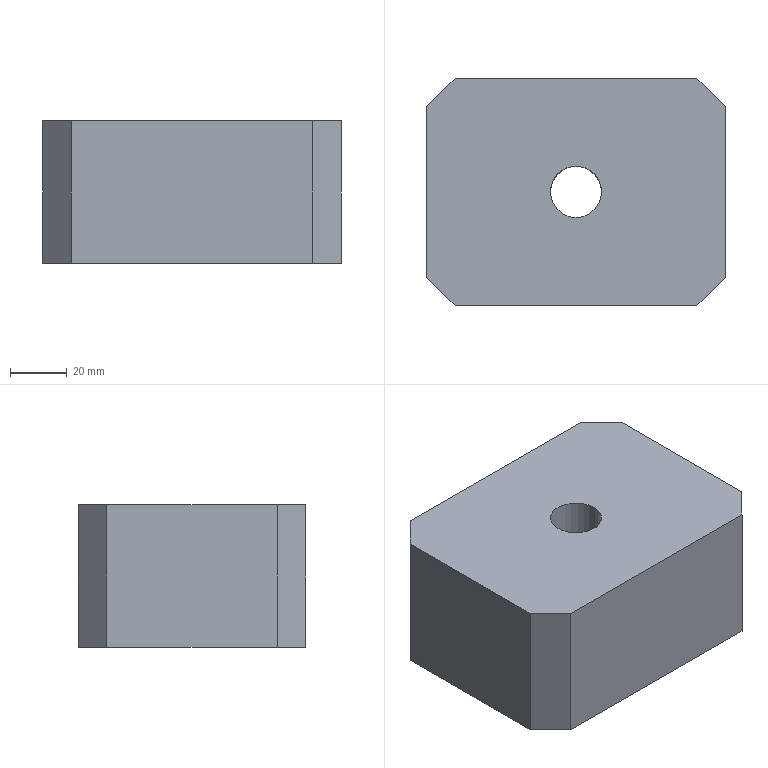Part | STEP file | [J453-EBZ05-16-00] | 1 solid | 12 faces | box 105 x 80 x 50 mm | volume 397277 mm3 | plane 10 | cylinder 2 | commonest cylinder face diameters 18 x2
STEP:
#1=CARTESIAN_POINT('',(0.,0.,0.));
#2=DIRECTION('',(0.,0.,1.));
#3=DIRECTION('',(1.,0.,0.));
#4=AXIS2_PLACEMENT_3D('',#1,#2,#3);
#5=CARTESIAN_POINT('',(61.5,40.,50.));
#6=VERTEX_POINT('',#5);
#7=CARTESIAN_POINT('',(61.5,40.,0.));
#8=VERTEX_POINT('',#7);
#9=CARTESIAN_POINT('',(61.5,40.,50.));
#10=DIRECTION('',(0.,0.,-1.));
#11=VECTOR('',#10,1.);
#12=LINE('',#9,#11);
#13=CARTESIAN_POINT('',(52.5,40.,50.));
#14=DIRECTION('',(0.,0.,-1.));
#15=DIRECTION('',(1.,0.,0.));
#16=AXIS2_PLACEMENT_3D('',#13,#14,#15);
#17=CYLINDRICAL_SURFACE('',#16,9.);
#18=CARTESIAN_POINT('',(6.283,0.));
#19=DIRECTION('',(0.,1.));
#20=VECTOR('',#19,1.);
#21=LINE('',#18,#20);
#22=(GEOMETRIC_REPRESENTATION_CONTEXT(2)PARAMETRIC_REPRESENTATION_CONTEXT()REPRESENTATION_CONTEXT('',''));
#23=DEFINITIONAL_REPRESENTATION('',(#21),#22);
#24=PCURVE('',#17,#23);
#25=CARTESIAN_POINT('',(52.5,40.,50.));
#26=DIRECTION('',(0.,0.,-1.));
#27=DIRECTION('',(1.,0.,0.));
#28=AXIS2_PLACEMENT_3D('',#25,#26,#27);
#29=CYLINDRICAL_SURFACE('',#28,9.);
#30=CARTESIAN_POINT('',(0.,0.));
#31=DIRECTION('',(0.,1.));
#32=VECTOR('',#31,1.);
#33=LINE('',#30,#32);
#34=(GEOMETRIC_REPRESENTATION_CONTEXT(2)PARAMETRIC_REPRESENTATION_CONTEXT()REPRESENTATION_CONTEXT('',''));
#35=DEFINITIONAL_REPRESENTATION('',(#33),#34);
#36=PCURVE('',#29,#35);
#37=SURFACE_CURVE('',#12,(#24,#36),.PCURVE_S1.);
#38=EDGE_CURVE('',#6,#8,#37,.T.);
#39=ORIENTED_EDGE('',*,*,#38,.T.);
#40=CARTESIAN_POINT('',(43.5,40.,0.));
#41=VERTEX_POINT('',#40);
#42=CARTESIAN_POINT('',(52.5,40.,0.));
#43=DIRECTION('',(0.,0.,1.));
#44=DIRECTION('',(-1.,0.,0.));
#45=AXIS2_PLACEMENT_3D('',#42,#43,#44);
#46=CIRCLE('',#45,9.);
#47=CARTESIAN_POINT('',(9.425,50.));
#48=DIRECTION('',(-1.,0.));
#49=VECTOR('',#48,1.);
#50=LINE('',#47,#49);
#51=(GEOMETRIC_REPRESENTATION_CONTEXT(2)PARAMETRIC_REPRESENTATION_CONTEXT()REPRESENTATION_CONTEXT('',''));
#52=DEFINITIONAL_REPRESENTATION('',(#50),#51);
#53=PCURVE('',#17,#52);
#54=CARTESIAN_POINT('',(0.,40.,0.));
#55=DIRECTION('',(0.,0.,-1.));
#56=DIRECTION('',(1.,0.,0.));
#57=AXIS2_PLACEMENT_3D('',#54,#55,#56);
#58=PLANE('',#57);
#59=CARTESIAN_POINT('',(43.5,0.));
#60=CARTESIAN_POINT('',(43.5,15.588));
#61=CARTESIAN_POINT('',(57.,7.794));
#62=CARTESIAN_POINT('',(70.5,0.));
#63=CARTESIAN_POINT('',(57.,-7.794));
#64=CARTESIAN_POINT('',(43.5,-15.588));
#65=CARTESIAN_POINT('',(43.5,0.));
#66=(BOUNDED_CURVE()B_SPLINE_CURVE(2,(#59,#60,#61,#62,#63,#64,#65),.UNSPECIFIED.,.T.,.F.)B_SPLINE_CURVE_WITH_KNOTS((1,2,2,2,2,1),(-2.094,0.,2.094,4.189,6.283,8.378),.UNSPECIFIED.)CURVE()GEOMETRIC_REPRESENTATION_ITEM()RATIONAL_B_SPLINE_CURVE((1.,0.5,1.,0.5,1.,0.5,1.))REPRESENTATION_ITEM(''));
#67=(GEOMETRIC_REPRESENTATION_CONTEXT(2)PARAMETRIC_REPRESENTATION_CONTEXT()REPRESENTATION_CONTEXT('',''));
#68=DEFINITIONAL_REPRESENTATION('',(#66),#67);
#69=PCURVE('',#58,#68);
#70=SURFACE_CURVE('',#46,(#53,#69),.PCURVE_S1.);
#71=EDGE_CURVE('',#8,#41,#70,.T.);
#72=ORIENTED_EDGE('',*,*,#71,.T.);
#73=CARTESIAN_POINT('',(43.5,40.,50.));
#74=VERTEX_POINT('',#73);
#75=CARTESIAN_POINT('',(43.5,40.,50.));
#76=DIRECTION('',(0.,0.,-1.));
#77=VECTOR('',#76,1.);
#78=LINE('',#75,#77);
#79=CARTESIAN_POINT('',(3.142,0.));
#80=DIRECTION('',(0.,1.));
#81=VECTOR('',#80,1.);
#82=LINE('',#79,#81);
#83=(GEOMETRIC_REPRESENTATION_CONTEXT(2)PARAMETRIC_REPRESENTATION_CONTEXT()REPRESENTATION_CONTEXT('',''));
#84=DEFINITIONAL_REPRESENTATION('',(#82),#83);
#85=PCURVE('',#17,#84);
#86=CARTESIAN_POINT('',(3.142,0.));
#87=DIRECTION('',(0.,1.));
#88=VECTOR('',#87,1.);
#89=LINE('',#86,#88);
#90=(GEOMETRIC_REPRESENTATION_CONTEXT(2)PARAMETRIC_REPRESENTATION_CONTEXT()REPRESENTATION_CONTEXT('',''));
#91=DEFINITIONAL_REPRESENTATION('',(#89),#90);
#92=PCURVE('',#29,#91);
#93=SURFACE_CURVE('',#78,(#85,#92),.PCURVE_S1.);
#94=EDGE_CURVE('',#74,#41,#93,.T.);
#95=ORIENTED_EDGE('',*,*,#94,.F.);
#96=CARTESIAN_POINT('',(52.5,40.,50.));
#97=DIRECTION('',(0.,0.,-1.));
#98=DIRECTION('',(1.,0.,0.));
#99=AXIS2_PLACEMENT_3D('',#96,#97,#98);
#100=CIRCLE('',#99,9.);
#101=CARTESIAN_POINT('',(0.,0.));
#102=DIRECTION('',(1.,0.));
#103=VECTOR('',#102,1.);
#104=LINE('',#101,#103);
#105=(GEOMETRIC_REPRESENTATION_CONTEXT(2)PARAMETRIC_REPRESENTATION_CONTEXT()REPRESENTATION_CONTEXT('',''));
#106=DEFINITIONAL_REPRESENTATION('',(#104),#105);
#107=PCURVE('',#17,#106);
#108=CARTESIAN_POINT('',(0.,40.,50.));
#109=DIRECTION('',(0.,0.,1.));
#110=DIRECTION('',(-1.,0.,0.));
#111=AXIS2_PLACEMENT_3D('',#108,#109,#110);
#112=PLANE('',#111);
#113=CARTESIAN_POINT('',(-61.5,0.));
#114=CARTESIAN_POINT('',(-61.5,15.588));
#115=CARTESIAN_POINT('',(-48.,7.794));
#116=CARTESIAN_POINT('',(-34.5,0.));
#117=CARTESIAN_POINT('',(-48.,-7.794));
#118=CARTESIAN_POINT('',(-61.5,-15.588));
#119=CARTESIAN_POINT('',(-61.5,0.));
#120=(BOUNDED_CURVE()B_SPLINE_CURVE(2,(#113,#114,#115,#116,#117,#118,#119),.UNSPECIFIED.,.T.,.F.)B_SPLINE_CURVE_WITH_KNOTS((1,2,2,2,2,1),(-2.094,0.,2.094,4.189,6.283,8.378),.UNSPECIFIED.)CURVE()GEOMETRIC_REPRESENTATION_ITEM()RATIONAL_B_SPLINE_CURVE((1.,0.5,1.,0.5,1.,0.5,1.))REPRESENTATION_ITEM(''));
#121=(GEOMETRIC_REPRESENTATION_CONTEXT(2)PARAMETRIC_REPRESENTATION_CONTEXT()REPRESENTATION_CONTEXT('',''));
#122=DEFINITIONAL_REPRESENTATION('',(#120),#121);
#123=PCURVE('',#112,#122);
#124=SURFACE_CURVE('',#100,(#107,#123),.PCURVE_S1.);
#125=EDGE_CURVE('',#74,#6,#124,.T.);
#126=ORIENTED_EDGE('',*,*,#125,.T.);
#127=EDGE_LOOP('',(#39,#72,#95,#126));
#128=FACE_BOUND('',#127,.F.);
#129=ADVANCED_FACE('',(#128),#17,.F.);
#130=CARTESIAN_POINT('',(105.,70.,0.));
#131=VERTEX_POINT('',#130);
#132=CARTESIAN_POINT('',(105.,10.,0.));
#133=VERTEX_POINT('',#132);
#134=CARTESIAN_POINT('',(105.,40.,0.));
#135=DIRECTION('',(0.,-1.,0.));
#136=VECTOR('',#135,1.);
#137=LINE('',#134,#136);
#138=CARTESIAN_POINT('',(105.,40.,25.));
#139=DIRECTION('',(1.,0.,0.));
#140=DIRECTION('',(0.,0.,1.));
#141=AXIS2_PLACEMENT_3D('',#138,#139,#140);
#142=PLANE('',#141);
#143=CARTESIAN_POINT('',(-25.,0.));
#144=DIRECTION('',(0.,1.));
#145=VECTOR('',#144,1.);
#146=LINE('',#143,#145);
#147=(GEOMETRIC_REPRESENTATION_CONTEXT(2)PARAMETRIC_REPRESENTATION_CONTEXT()REPRESENTATION_CONTEXT('',''));
#148=DEFINITIONAL_REPRESENTATION('',(#146),#147);
#149=PCURVE('',#142,#148);
#150=CARTESIAN_POINT('',(105.,0.));
#151=DIRECTION('',(0.,1.));
#152=VECTOR('',#151,1.);
#153=LINE('',#150,#152);
#154=(GEOMETRIC_REPRESENTATION_CONTEXT(2)PARAMETRIC_REPRESENTATION_CONTEXT()REPRESENTATION_CONTEXT('',''));
#155=DEFINITIONAL_REPRESENTATION('',(#153),#154);
#156=PCURVE('',#58,#155);
#157=SURFACE_CURVE('',#137,(#149,#156),.PCURVE_S1.);
#158=EDGE_CURVE('',#131,#133,#157,.T.);
#159=ORIENTED_EDGE('',*,*,#158,.F.);
#160=CARTESIAN_POINT('',(105.,70.,50.));
#161=VERTEX_POINT('',#160);
#162=CARTESIAN_POINT('',(105.,70.,25.));
#163=DIRECTION('',(0.,0.,1.));
#164=VECTOR('',#163,1.);
#165=LINE('',#162,#164);
#166=CARTESIAN_POINT('',(0.,-30.));
#167=DIRECTION('',(1.,0.));
#168=VECTOR('',#167,1.);
#169=LINE('',#166,#168);
#170=(GEOMETRIC_REPRESENTATION_CONTEXT(2)PARAMETRIC_REPRESENTATION_CONTEXT()REPRESENTATION_CONTEXT('',''));
#171=DEFINITIONAL_REPRESENTATION('',(#169),#170);
#172=PCURVE('',#142,#171);
#173=CARTESIAN_POINT('',(95.,80.,25.));
#174=DIRECTION('',(-0.7071,-0.7071,0.));
#175=DIRECTION('',(0.,0.,-1.));
#176=AXIS2_PLACEMENT_3D('',#173,#174,#175);
#177=PLANE('',#176);
#178=CARTESIAN_POINT('',(0.,14.142));
#179=DIRECTION('',(-1.,0.));
#180=VECTOR('',#179,1.);
#181=LINE('',#178,#180);
#182=(GEOMETRIC_REPRESENTATION_CONTEXT(2)PARAMETRIC_REPRESENTATION_CONTEXT()REPRESENTATION_CONTEXT('',''));
#183=DEFINITIONAL_REPRESENTATION('',(#181),#182);
#184=PCURVE('',#177,#183);
#185=SURFACE_CURVE('',#165,(#172,#184),.PCURVE_S1.);
#186=EDGE_CURVE('',#131,#161,#185,.T.);
#187=ORIENTED_EDGE('',*,*,#186,.T.);
#188=CARTESIAN_POINT('',(105.,10.,50.));
#189=VERTEX_POINT('',#188);
#190=CARTESIAN_POINT('',(105.,40.,50.));
#191=DIRECTION('',(0.,1.,0.));
#192=VECTOR('',#191,1.);
#193=LINE('',#190,#192);
#194=CARTESIAN_POINT('',(25.,0.));
#195=DIRECTION('',(0.,-1.));
#196=VECTOR('',#195,1.);
#197=LINE('',#194,#196);
#198=(GEOMETRIC_REPRESENTATION_CONTEXT(2)PARAMETRIC_REPRESENTATION_CONTEXT()REPRESENTATION_CONTEXT('',''));
#199=DEFINITIONAL_REPRESENTATION('',(#197),#198);
#200=PCURVE('',#142,#199);
#201=CARTESIAN_POINT('',(-105.,0.));
#202=DIRECTION('',(0.,-1.));
#203=VECTOR('',#202,1.);
#204=LINE('',#201,#203);
#205=(GEOMETRIC_REPRESENTATION_CONTEXT(2)PARAMETRIC_REPRESENTATION_CONTEXT()REPRESENTATION_CONTEXT('',''));
#206=DEFINITIONAL_REPRESENTATION('',(#204),#205);
#207=PCURVE('',#112,#206);
#208=SURFACE_CURVE('',#193,(#200,#207),.PCURVE_S1.);
#209=EDGE_CURVE('',#189,#161,#208,.T.);
#210=ORIENTED_EDGE('',*,*,#209,.F.);
#211=CARTESIAN_POINT('',(105.,10.,25.));
#212=DIRECTION('',(0.,0.,-1.));
#213=VECTOR('',#212,1.);
#214=LINE('',#211,#213);
#215=CARTESIAN_POINT('',(0.,30.));
#216=DIRECTION('',(-1.,0.));
#217=VECTOR('',#216,1.);
#218=LINE('',#215,#217);
#219=(GEOMETRIC_REPRESENTATION_CONTEXT(2)PARAMETRIC_REPRESENTATION_CONTEXT()REPRESENTATION_CONTEXT('',''));
#220=DEFINITIONAL_REPRESENTATION('',(#218),#219);
#221=PCURVE('',#142,#220);
#222=CARTESIAN_POINT('',(95.,0.,25.));
#223=DIRECTION('',(-0.7071,0.7071,0.));
#224=DIRECTION('',(0.,0.,1.));
#225=AXIS2_PLACEMENT_3D('',#222,#223,#224);
#226=PLANE('',#225);
#227=CARTESIAN_POINT('',(0.,14.142));
#228=DIRECTION('',(-1.,0.));
#229=VECTOR('',#228,1.);
#230=LINE('',#227,#229);
#231=(GEOMETRIC_REPRESENTATION_CONTEXT(2)PARAMETRIC_REPRESENTATION_CONTEXT()REPRESENTATION_CONTEXT('',''));
#232=DEFINITIONAL_REPRESENTATION('',(#230),#231);
#233=PCURVE('',#226,#232);
#234=SURFACE_CURVE('',#214,(#221,#233),.PCURVE_S1.);
#235=EDGE_CURVE('',#189,#133,#234,.T.);
#236=ORIENTED_EDGE('',*,*,#235,.T.);
#237=EDGE_LOOP('',(#159,#187,#210,#236));
#238=FACE_BOUND('',#237,.T.);
#239=ADVANCED_FACE('',(#238),#142,.T.);
#240=CARTESIAN_POINT('',(10.,80.,50.));
#241=VERTEX_POINT('',#240);
#242=CARTESIAN_POINT('',(95.,80.,50.));
#243=VERTEX_POINT('',#242);
#244=CARTESIAN_POINT('',(0.,80.,50.));
#245=DIRECTION('',(1.,0.,0.));
#246=VECTOR('',#245,1.);
#247=LINE('',#244,#246);
#248=CARTESIAN_POINT('',(0.,80.,25.));
#249=DIRECTION('',(0.,1.,0.));
#250=DIRECTION('',(-1.,0.,0.));
#251=AXIS2_PLACEMENT_3D('',#248,#249,#250);
#252=PLANE('',#251);
#253=CARTESIAN_POINT('',(0.,25.));
#254=DIRECTION('',(-1.,0.));
#255=VECTOR('',#254,1.);
#256=LINE('',#253,#255);
#257=(GEOMETRIC_REPRESENTATION_CONTEXT(2)PARAMETRIC_REPRESENTATION_CONTEXT()REPRESENTATION_CONTEXT('',''));
#258=DEFINITIONAL_REPRESENTATION('',(#256),#257);
#259=PCURVE('',#252,#258);
#260=CARTESIAN_POINT('',(0.,-40.));
#261=DIRECTION('',(-1.,0.));
#262=VECTOR('',#261,1.);
#263=LINE('',#260,#262);
#264=(GEOMETRIC_REPRESENTATION_CONTEXT(2)PARAMETRIC_REPRESENTATION_CONTEXT()REPRESENTATION_CONTEXT('',''));
#265=DEFINITIONAL_REPRESENTATION('',(#263),#264);
#266=PCURVE('',#112,#265);
#267=SURFACE_CURVE('',#247,(#259,#266),.PCURVE_S1.);
#268=EDGE_CURVE('',#241,#243,#267,.T.);
#269=ORIENTED_EDGE('',*,*,#268,.T.);
#270=CARTESIAN_POINT('',(95.,80.,0.));
#271=VERTEX_POINT('',#270);
#272=CARTESIAN_POINT('',(95.,80.,25.));
#273=DIRECTION('',(0.,0.,-1.));
#274=VECTOR('',#273,1.);
#275=LINE('',#272,#274);
#276=CARTESIAN_POINT('',(-95.,0.));
#277=DIRECTION('',(0.,-1.));
#278=VECTOR('',#277,1.);
#279=LINE('',#276,#278);
#280=(GEOMETRIC_REPRESENTATION_CONTEXT(2)PARAMETRIC_REPRESENTATION_CONTEXT()REPRESENTATION_CONTEXT('',''));
#281=DEFINITIONAL_REPRESENTATION('',(#279),#280);
#282=PCURVE('',#252,#281);
#283=CARTESIAN_POINT('',(0.,0.));
#284=DIRECTION('',(1.,0.));
#285=VECTOR('',#284,1.);
#286=LINE('',#283,#285);
#287=(GEOMETRIC_REPRESENTATION_CONTEXT(2)PARAMETRIC_REPRESENTATION_CONTEXT()REPRESENTATION_CONTEXT('',''));
#288=DEFINITIONAL_REPRESENTATION('',(#286),#287);
#289=PCURVE('',#177,#288);
#290=SURFACE_CURVE('',#275,(#282,#289),.PCURVE_S1.);
#291=EDGE_CURVE('',#243,#271,#290,.T.);
#292=ORIENTED_EDGE('',*,*,#291,.T.);
#293=CARTESIAN_POINT('',(10.,80.,0.));
#294=VERTEX_POINT('',#293);
#295=CARTESIAN_POINT('',(0.,80.,0.));
#296=DIRECTION('',(1.,0.,0.));
#297=VECTOR('',#296,1.);
#298=LINE('',#295,#297);
#299=CARTESIAN_POINT('',(0.,-25.));
#300=DIRECTION('',(-1.,0.));
#301=VECTOR('',#300,1.);
#302=LINE('',#299,#301);
#303=(GEOMETRIC_REPRESENTATION_CONTEXT(2)PARAMETRIC_REPRESENTATION_CONTEXT()REPRESENTATION_CONTEXT('',''));
#304=DEFINITIONAL_REPRESENTATION('',(#302),#303);
#305=PCURVE('',#252,#304);
#306=CARTESIAN_POINT('',(0.,-40.));
#307=DIRECTION('',(1.,0.));
#308=VECTOR('',#307,1.);
#309=LINE('',#306,#308);
#310=(GEOMETRIC_REPRESENTATION_CONTEXT(2)PARAMETRIC_REPRESENTATION_CONTEXT()REPRESENTATION_CONTEXT('',''));
#311=DEFINITIONAL_REPRESENTATION('',(#309),#310);
#312=PCURVE('',#58,#311);
#313=SURFACE_CURVE('',#298,(#305,#312),.PCURVE_S1.);
#314=EDGE_CURVE('',#294,#271,#313,.T.);
#315=ORIENTED_EDGE('',*,*,#314,.F.);
#316=CARTESIAN_POINT('',(10.,80.,25.));
#317=DIRECTION('',(0.,0.,1.));
#318=VECTOR('',#317,1.);
#319=LINE('',#316,#318);
#320=CARTESIAN_POINT('',(-10.,0.));
#321=DIRECTION('',(0.,1.));
#322=VECTOR('',#321,1.);
#323=LINE('',#320,#322);
#324=(GEOMETRIC_REPRESENTATION_CONTEXT(2)PARAMETRIC_REPRESENTATION_CONTEXT()REPRESENTATION_CONTEXT('',''));
#325=DEFINITIONAL_REPRESENTATION('',(#323),#324);
#326=PCURVE('',#252,#325);
#327=CARTESIAN_POINT('',(10.,80.,25.));
#328=DIRECTION('',(0.7071,-0.7071,0.));
#329=DIRECTION('',(0.,0.,1.));
#330=AXIS2_PLACEMENT_3D('',#327,#328,#329);
#331=PLANE('',#330);
#332=CARTESIAN_POINT('',(0.,0.));
#333=DIRECTION('',(1.,0.));
#334=VECTOR('',#333,1.);
#335=LINE('',#332,#334);
#336=(GEOMETRIC_REPRESENTATION_CONTEXT(2)PARAMETRIC_REPRESENTATION_CONTEXT()REPRESENTATION_CONTEXT('',''));
#337=DEFINITIONAL_REPRESENTATION('',(#335),#336);
#338=PCURVE('',#331,#337);
#339=SURFACE_CURVE('',#319,(#326,#338),.PCURVE_S1.);
#340=EDGE_CURVE('',#294,#241,#339,.T.);
#341=ORIENTED_EDGE('',*,*,#340,.T.);
#342=EDGE_LOOP('',(#269,#292,#315,#341));
#343=FACE_BOUND('',#342,.T.);
#344=ADVANCED_FACE('',(#343),#252,.T.);
#345=ORIENTED_EDGE('',*,*,#71,.T.);
#346=CARTESIAN_POINT('',(52.5,40.,0.));
#347=DIRECTION('',(0.,0.,1.));
#348=DIRECTION('',(-1.,0.,0.));
#349=AXIS2_PLACEMENT_3D('',#346,#347,#348);
#350=CIRCLE('',#349,9.);
#351=CARTESIAN_POINT('',(43.5,0.));
#352=CARTESIAN_POINT('',(43.5,15.588));
#353=CARTESIAN_POINT('',(57.,7.794));
#354=CARTESIAN_POINT('',(70.5,0.));
#355=CARTESIAN_POINT('',(57.,-7.794));
#356=CARTESIAN_POINT('',(43.5,-15.588));
#357=CARTESIAN_POINT('',(43.5,0.));
#358=(BOUNDED_CURVE()B_SPLINE_CURVE(2,(#351,#352,#353,#354,#355,#356,#357),.UNSPECIFIED.,.T.,.F.)B_SPLINE_CURVE_WITH_KNOTS((1,2,2,2,2,1),(-2.094,0.,2.094,4.189,6.283,8.378),.UNSPECIFIED.)CURVE()GEOMETRIC_REPRESENTATION_ITEM()RATIONAL_B_SPLINE_CURVE((1.,0.5,1.,0.5,1.,0.5,1.))REPRESENTATION_ITEM(''));
#359=(GEOMETRIC_REPRESENTATION_CONTEXT(2)PARAMETRIC_REPRESENTATION_CONTEXT()REPRESENTATION_CONTEXT('',''));
#360=DEFINITIONAL_REPRESENTATION('',(#358),#359);
#361=PCURVE('',#58,#360);
#362=CARTESIAN_POINT('',(3.142,50.));
#363=DIRECTION('',(-1.,0.));
#364=VECTOR('',#363,1.);
#365=LINE('',#362,#364);
#366=(GEOMETRIC_REPRESENTATION_CONTEXT(2)PARAMETRIC_REPRESENTATION_CONTEXT()REPRESENTATION_CONTEXT('',''));
#367=DEFINITIONAL_REPRESENTATION('',(#365),#366);
#368=PCURVE('',#29,#367);
#369=SURFACE_CURVE('',#350,(#361,#368),.PCURVE_S1.);
#370=EDGE_CURVE('',#41,#8,#369,.T.);
#371=ORIENTED_EDGE('',*,*,#370,.T.);
#372=EDGE_LOOP('',(#345,#371));
#373=FACE_BOUND('',#372,.T.);
#374=ORIENTED_EDGE('',*,*,#314,.T.);
#375=CARTESIAN_POINT('',(67.5,107.5,0.));
#376=DIRECTION('',(0.7071,-0.7071,0.));
#377=VECTOR('',#376,1.);
#378=LINE('',#375,#377);
#379=CARTESIAN_POINT('',(67.5,-67.5));
#380=DIRECTION('',(0.7071,0.7071));
#381=VECTOR('',#380,1.);
#382=LINE('',#379,#381);
#383=(GEOMETRIC_REPRESENTATION_CONTEXT(2)PARAMETRIC_REPRESENTATION_CONTEXT()REPRESENTATION_CONTEXT('',''));
#384=DEFINITIONAL_REPRESENTATION('',(#382),#383);
#385=PCURVE('',#58,#384);
#386=CARTESIAN_POINT('',(25.,-38.891));
#387=DIRECTION('',(0.,1.));
#388=VECTOR('',#387,1.);
#389=LINE('',#386,#388);
#390=(GEOMETRIC_REPRESENTATION_CONTEXT(2)PARAMETRIC_REPRESENTATION_CONTEXT()REPRESENTATION_CONTEXT('',''));
#391=DEFINITIONAL_REPRESENTATION('',(#389),#390);
#392=PCURVE('',#177,#391);
#393=SURFACE_CURVE('',#378,(#385,#392),.PCURVE_S1.);
#394=EDGE_CURVE('',#271,#131,#393,.T.);
#395=ORIENTED_EDGE('',*,*,#394,.T.);
#396=ORIENTED_EDGE('',*,*,#158,.T.);
#397=CARTESIAN_POINT('',(95.,0.,0.));
#398=VERTEX_POINT('',#397);
#399=CARTESIAN_POINT('',(67.5,-27.5,0.));
#400=DIRECTION('',(-0.7071,-0.7071,0.));
#401=VECTOR('',#400,1.);
#402=LINE('',#399,#401);
#403=CARTESIAN_POINT('',(67.5,67.5));
#404=DIRECTION('',(-0.7071,0.7071));
#405=VECTOR('',#404,1.);
#406=LINE('',#403,#405);
#407=(GEOMETRIC_REPRESENTATION_CONTEXT(2)PARAMETRIC_REPRESENTATION_CONTEXT()REPRESENTATION_CONTEXT('',''));
#408=DEFINITIONAL_REPRESENTATION('',(#406),#407);
#409=PCURVE('',#58,#408);
#410=CARTESIAN_POINT('',(-25.,-38.891));
#411=DIRECTION('',(0.,-1.));
#412=VECTOR('',#411,1.);
#413=LINE('',#410,#412);
#414=(GEOMETRIC_REPRESENTATION_CONTEXT(2)PARAMETRIC_REPRESENTATION_CONTEXT()REPRESENTATION_CONTEXT('',''));
#415=DEFINITIONAL_REPRESENTATION('',(#413),#414);
#416=PCURVE('',#226,#415);
#417=SURFACE_CURVE('',#402,(#409,#416),.PCURVE_S1.);
#418=EDGE_CURVE('',#133,#398,#417,.T.);
#419=ORIENTED_EDGE('',*,*,#418,.T.);
#420=CARTESIAN_POINT('',(10.,0.,0.));
#421=VERTEX_POINT('',#420);
#422=CARTESIAN_POINT('',(0.,0.,0.));
#423=DIRECTION('',(1.,0.,0.));
#424=VECTOR('',#423,1.);
#425=LINE('',#422,#424);
#426=CARTESIAN_POINT('',(0.,40.));
#427=DIRECTION('',(1.,0.));
#428=VECTOR('',#427,1.);
#429=LINE('',#426,#428);
#430=(GEOMETRIC_REPRESENTATION_CONTEXT(2)PARAMETRIC_REPRESENTATION_CONTEXT()REPRESENTATION_CONTEXT('',''));
#431=DEFINITIONAL_REPRESENTATION('',(#429),#430);
#432=PCURVE('',#58,#431);
#433=CARTESIAN_POINT('',(0.,0.,25.));
#434=DIRECTION('',(0.,-1.,0.));
#435=DIRECTION('',(1.,0.,0.));
#436=AXIS2_PLACEMENT_3D('',#433,#434,#435);
#437=PLANE('',#436);
#438=CARTESIAN_POINT('',(0.,-25.));
#439=DIRECTION('',(1.,0.));
#440=VECTOR('',#439,1.);
#441=LINE('',#438,#440);
#442=(GEOMETRIC_REPRESENTATION_CONTEXT(2)PARAMETRIC_REPRESENTATION_CONTEXT()REPRESENTATION_CONTEXT('',''));
#443=DEFINITIONAL_REPRESENTATION('',(#441),#442);
#444=PCURVE('',#437,#443);
#445=SURFACE_CURVE('',#425,(#432,#444),.PCURVE_S1.);
#446=EDGE_CURVE('',#421,#398,#445,.T.);
#447=ORIENTED_EDGE('',*,*,#446,.F.);
#448=CARTESIAN_POINT('',(0.,10.,0.));
#449=VERTEX_POINT('',#448);
#450=CARTESIAN_POINT('',(-15.,25.,0.));
#451=DIRECTION('',(-0.7071,0.7071,0.));
#452=VECTOR('',#451,1.);
#453=LINE('',#450,#452);
#454=CARTESIAN_POINT('',(-15.,15.));
#455=DIRECTION('',(-0.7071,-0.7071));
#456=VECTOR('',#455,1.);
#457=LINE('',#454,#456);
#458=(GEOMETRIC_REPRESENTATION_CONTEXT(2)PARAMETRIC_REPRESENTATION_CONTEXT()REPRESENTATION_CONTEXT('',''));
#459=DEFINITIONAL_REPRESENTATION('',(#457),#458);
#460=PCURVE('',#58,#459);
#461=CARTESIAN_POINT('',(10.,0.,25.));
#462=DIRECTION('',(0.7071,0.7071,0.));
#463=DIRECTION('',(0.,0.,-1.));
#464=AXIS2_PLACEMENT_3D('',#461,#462,#463);
#465=PLANE('',#464);
#466=CARTESIAN_POINT('',(25.,35.355));
#467=DIRECTION('',(0.,1.));
#468=VECTOR('',#467,1.);
#469=LINE('',#466,#468);
#470=(GEOMETRIC_REPRESENTATION_CONTEXT(2)PARAMETRIC_REPRESENTATION_CONTEXT()REPRESENTATION_CONTEXT('',''));
#471=DEFINITIONAL_REPRESENTATION('',(#469),#470);
#472=PCURVE('',#465,#471);
#473=SURFACE_CURVE('',#453,(#460,#472),.PCURVE_S1.);
#474=EDGE_CURVE('',#421,#449,#473,.T.);
#475=ORIENTED_EDGE('',*,*,#474,.T.);
#476=CARTESIAN_POINT('',(0.,70.,0.));
#477=VERTEX_POINT('',#476);
#478=CARTESIAN_POINT('',(0.,40.,0.));
#479=DIRECTION('',(0.,1.,0.));
#480=VECTOR('',#479,1.);
#481=LINE('',#478,#480);
#482=CARTESIAN_POINT('',(0.,0.));
#483=DIRECTION('',(0.,-1.));
#484=VECTOR('',#483,1.);
#485=LINE('',#482,#484);
#486=(GEOMETRIC_REPRESENTATION_CONTEXT(2)PARAMETRIC_REPRESENTATION_CONTEXT()REPRESENTATION_CONTEXT('',''));
#487=DEFINITIONAL_REPRESENTATION('',(#485),#486);
#488=PCURVE('',#58,#487);
#489=CARTESIAN_POINT('',(0.,40.,25.));
#490=DIRECTION('',(-1.,0.,0.));
#491=DIRECTION('',(0.,0.,-1.));
#492=AXIS2_PLACEMENT_3D('',#489,#490,#491);
#493=PLANE('',#492);
#494=CARTESIAN_POINT('',(25.,0.));
#495=DIRECTION('',(0.,-1.));
#496=VECTOR('',#495,1.);
#497=LINE('',#494,#496);
#498=(GEOMETRIC_REPRESENTATION_CONTEXT(2)PARAMETRIC_REPRESENTATION_CONTEXT()REPRESENTATION_CONTEXT('',''));
#499=DEFINITIONAL_REPRESENTATION('',(#497),#498);
#500=PCURVE('',#493,#499);
#501=SURFACE_CURVE('',#481,(#488,#500),.PCURVE_S1.);
#502=EDGE_CURVE('',#449,#477,#501,.T.);
#503=ORIENTED_EDGE('',*,*,#502,.T.);
#504=CARTESIAN_POINT('',(-15.,55.,0.));
#505=DIRECTION('',(0.7071,0.7071,0.));
#506=VECTOR('',#505,1.);
#507=LINE('',#504,#506);
#508=CARTESIAN_POINT('',(-15.,-15.));
#509=DIRECTION('',(0.7071,-0.7071));
#510=VECTOR('',#509,1.);
#511=LINE('',#508,#510);
#512=(GEOMETRIC_REPRESENTATION_CONTEXT(2)PARAMETRIC_REPRESENTATION_CONTEXT()REPRESENTATION_CONTEXT('',''));
#513=DEFINITIONAL_REPRESENTATION('',(#511),#512);
#514=PCURVE('',#58,#513);
#515=CARTESIAN_POINT('',(-25.,35.355));
#516=DIRECTION('',(0.,-1.));
#517=VECTOR('',#516,1.);
#518=LINE('',#515,#517);
#519=(GEOMETRIC_REPRESENTATION_CONTEXT(2)PARAMETRIC_REPRESENTATION_CONTEXT()REPRESENTATION_CONTEXT('',''));
#520=DEFINITIONAL_REPRESENTATION('',(#518),#519);
#521=PCURVE('',#331,#520);
#522=SURFACE_CURVE('',#507,(#514,#521),.PCURVE_S1.);
#523=EDGE_CURVE('',#477,#294,#522,.T.);
#524=ORIENTED_EDGE('',*,*,#523,.T.);
#525=EDGE_LOOP('',(#374,#395,#396,#419,#447,#475,#503,#524));
#526=FACE_BOUND('',#525,.T.);
#527=ADVANCED_FACE('',(#373,#526),#58,.T.);
#528=ORIENTED_EDGE('',*,*,#446,.T.);
#529=CARTESIAN_POINT('',(95.,0.,50.));
#530=VERTEX_POINT('',#529);
#531=CARTESIAN_POINT('',(95.,0.,25.));
#532=DIRECTION('',(0.,0.,1.));
#533=VECTOR('',#532,1.);
#534=LINE('',#531,#533);
#535=CARTESIAN_POINT('',(95.,0.));
#536=DIRECTION('',(0.,1.));
#537=VECTOR('',#536,1.);
#538=LINE('',#535,#537);
#539=(GEOMETRIC_REPRESENTATION_CONTEXT(2)PARAMETRIC_REPRESENTATION_CONTEXT()REPRESENTATION_CONTEXT('',''));
#540=DEFINITIONAL_REPRESENTATION('',(#538),#539);
#541=PCURVE('',#437,#540);
#542=CARTESIAN_POINT('',(0.,0.));
#543=DIRECTION('',(1.,0.));
#544=VECTOR('',#543,1.);
#545=LINE('',#542,#544);
#546=(GEOMETRIC_REPRESENTATION_CONTEXT(2)PARAMETRIC_REPRESENTATION_CONTEXT()REPRESENTATION_CONTEXT('',''));
#547=DEFINITIONAL_REPRESENTATION('',(#545),#546);
#548=PCURVE('',#226,#547);
#549=SURFACE_CURVE('',#534,(#541,#548),.PCURVE_S1.);
#550=EDGE_CURVE('',#398,#530,#549,.T.);
#551=ORIENTED_EDGE('',*,*,#550,.T.);
#552=CARTESIAN_POINT('',(10.,0.,50.));
#553=VERTEX_POINT('',#552);
#554=CARTESIAN_POINT('',(0.,0.,50.));
#555=DIRECTION('',(1.,0.,0.));
#556=VECTOR('',#555,1.);
#557=LINE('',#554,#556);
#558=CARTESIAN_POINT('',(0.,25.));
#559=DIRECTION('',(1.,0.));
#560=VECTOR('',#559,1.);
#561=LINE('',#558,#560);
#562=(GEOMETRIC_REPRESENTATION_CONTEXT(2)PARAMETRIC_REPRESENTATION_CONTEXT()REPRESENTATION_CONTEXT('',''));
#563=DEFINITIONAL_REPRESENTATION('',(#561),#562);
#564=PCURVE('',#437,#563);
#565=CARTESIAN_POINT('',(0.,40.));
#566=DIRECTION('',(-1.,0.));
#567=VECTOR('',#566,1.);
#568=LINE('',#565,#567);
#569=(GEOMETRIC_REPRESENTATION_CONTEXT(2)PARAMETRIC_REPRESENTATION_CONTEXT()REPRESENTATION_CONTEXT('',''));
#570=DEFINITIONAL_REPRESENTATION('',(#568),#569);
#571=PCURVE('',#112,#570);
#572=SURFACE_CURVE('',#557,(#564,#571),.PCURVE_S1.);
#573=EDGE_CURVE('',#553,#530,#572,.T.);
#574=ORIENTED_EDGE('',*,*,#573,.F.);
#575=CARTESIAN_POINT('',(10.,0.,25.));
#576=DIRECTION('',(0.,0.,-1.));
#577=VECTOR('',#576,1.);
#578=LINE('',#575,#577);
#579=CARTESIAN_POINT('',(10.,0.));
#580=DIRECTION('',(0.,-1.));
#581=VECTOR('',#580,1.);
#582=LINE('',#579,#581);
#583=(GEOMETRIC_REPRESENTATION_CONTEXT(2)PARAMETRIC_REPRESENTATION_CONTEXT()REPRESENTATION_CONTEXT('',''));
#584=DEFINITIONAL_REPRESENTATION('',(#582),#583);
#585=PCURVE('',#437,#584);
#586=CARTESIAN_POINT('',(0.,0.));
#587=DIRECTION('',(1.,0.));
#588=VECTOR('',#587,1.);
#589=LINE('',#586,#588);
#590=(GEOMETRIC_REPRESENTATION_CONTEXT(2)PARAMETRIC_REPRESENTATION_CONTEXT()REPRESENTATION_CONTEXT('',''));
#591=DEFINITIONAL_REPRESENTATION('',(#589),#590);
#592=PCURVE('',#465,#591);
#593=SURFACE_CURVE('',#578,(#585,#592),.PCURVE_S1.);
#594=EDGE_CURVE('',#553,#421,#593,.T.);
#595=ORIENTED_EDGE('',*,*,#594,.T.);
#596=EDGE_LOOP('',(#528,#551,#574,#595));
#597=FACE_BOUND('',#596,.T.);
#598=ADVANCED_FACE('',(#597),#437,.T.);
#599=CARTESIAN_POINT('',(0.,70.,50.));
#600=VERTEX_POINT('',#599);
#601=CARTESIAN_POINT('',(0.,10.,50.));
#602=VERTEX_POINT('',#601);
#603=CARTESIAN_POINT('',(0.,40.,50.));
#604=DIRECTION('',(0.,-1.,0.));
#605=VECTOR('',#604,1.);
#606=LINE('',#603,#605);
#607=CARTESIAN_POINT('',(-25.,0.));
#608=DIRECTION('',(0.,1.));
#609=VECTOR('',#608,1.);
#610=LINE('',#607,#609);
#611=(GEOMETRIC_REPRESENTATION_CONTEXT(2)PARAMETRIC_REPRESENTATION_CONTEXT()REPRESENTATION_CONTEXT('',''));
#612=DEFINITIONAL_REPRESENTATION('',(#610),#611);
#613=PCURVE('',#493,#612);
#614=CARTESIAN_POINT('',(0.,0.));
#615=DIRECTION('',(0.,1.));
#616=VECTOR('',#615,1.);
#617=LINE('',#614,#616);
#618=(GEOMETRIC_REPRESENTATION_CONTEXT(2)PARAMETRIC_REPRESENTATION_CONTEXT()REPRESENTATION_CONTEXT('',''));
#619=DEFINITIONAL_REPRESENTATION('',(#617),#618);
#620=PCURVE('',#112,#619);
#621=SURFACE_CURVE('',#606,(#613,#620),.PCURVE_S1.);
#622=EDGE_CURVE('',#600,#602,#621,.T.);
#623=ORIENTED_EDGE('',*,*,#622,.F.);
#624=CARTESIAN_POINT('',(0.,70.,25.));
#625=DIRECTION('',(0.,0.,-1.));
#626=VECTOR('',#625,1.);
#627=LINE('',#624,#626);
#628=CARTESIAN_POINT('',(0.,-30.));
#629=DIRECTION('',(1.,0.));
#630=VECTOR('',#629,1.);
#631=LINE('',#628,#630);
#632=(GEOMETRIC_REPRESENTATION_CONTEXT(2)PARAMETRIC_REPRESENTATION_CONTEXT()REPRESENTATION_CONTEXT('',''));
#633=DEFINITIONAL_REPRESENTATION('',(#631),#632);
#634=PCURVE('',#493,#633);
#635=CARTESIAN_POINT('',(0.,14.142));
#636=DIRECTION('',(-1.,0.));
#637=VECTOR('',#636,1.);
#638=LINE('',#635,#637);
#639=(GEOMETRIC_REPRESENTATION_CONTEXT(2)PARAMETRIC_REPRESENTATION_CONTEXT()REPRESENTATION_CONTEXT('',''));
#640=DEFINITIONAL_REPRESENTATION('',(#638),#639);
#641=PCURVE('',#331,#640);
#642=SURFACE_CURVE('',#627,(#634,#641),.PCURVE_S1.);
#643=EDGE_CURVE('',#600,#477,#642,.T.);
#644=ORIENTED_EDGE('',*,*,#643,.T.);
#645=ORIENTED_EDGE('',*,*,#502,.F.);
#646=CARTESIAN_POINT('',(0.,10.,25.));
#647=DIRECTION('',(0.,0.,1.));
#648=VECTOR('',#647,1.);
#649=LINE('',#646,#648);
#650=CARTESIAN_POINT('',(0.,30.));
#651=DIRECTION('',(-1.,0.));
#652=VECTOR('',#651,1.);
#653=LINE('',#650,#652);
#654=(GEOMETRIC_REPRESENTATION_CONTEXT(2)PARAMETRIC_REPRESENTATION_CONTEXT()REPRESENTATION_CONTEXT('',''));
#655=DEFINITIONAL_REPRESENTATION('',(#653),#654);
#656=PCURVE('',#493,#655);
#657=CARTESIAN_POINT('',(0.,14.142));
#658=DIRECTION('',(-1.,0.));
#659=VECTOR('',#658,1.);
#660=LINE('',#657,#659);
#661=(GEOMETRIC_REPRESENTATION_CONTEXT(2)PARAMETRIC_REPRESENTATION_CONTEXT()REPRESENTATION_CONTEXT('',''));
#662=DEFINITIONAL_REPRESENTATION('',(#660),#661);
#663=PCURVE('',#465,#662);
#664=SURFACE_CURVE('',#649,(#656,#663),.PCURVE_S1.);
#665=EDGE_CURVE('',#449,#602,#664,.T.);
#666=ORIENTED_EDGE('',*,*,#665,.T.);
#667=EDGE_LOOP('',(#623,#644,#645,#666));
#668=FACE_BOUND('',#667,.T.);
#669=ADVANCED_FACE('',(#668),#493,.T.);
#670=CARTESIAN_POINT('',(52.5,40.,50.));
#671=DIRECTION('',(0.,0.,-1.));
#672=DIRECTION('',(1.,0.,0.));
#673=AXIS2_PLACEMENT_3D('',#670,#671,#672);
#674=CIRCLE('',#673,9.);
#675=CARTESIAN_POINT('',(-61.5,0.));
#676=CARTESIAN_POINT('',(-61.5,15.588));
#677=CARTESIAN_POINT('',(-48.,7.794));
#678=CARTESIAN_POINT('',(-34.5,0.));
#679=CARTESIAN_POINT('',(-48.,-7.794));
#680=CARTESIAN_POINT('',(-61.5,-15.588));
#681=CARTESIAN_POINT('',(-61.5,0.));
#682=(BOUNDED_CURVE()B_SPLINE_CURVE(2,(#675,#676,#677,#678,#679,#680,#681),.UNSPECIFIED.,.T.,.F.)B_SPLINE_CURVE_WITH_KNOTS((1,2,2,2,2,1),(-2.094,0.,2.094,4.189,6.283,8.378),.UNSPECIFIED.)CURVE()GEOMETRIC_REPRESENTATION_ITEM()RATIONAL_B_SPLINE_CURVE((1.,0.5,1.,0.5,1.,0.5,1.))REPRESENTATION_ITEM(''));
#683=(GEOMETRIC_REPRESENTATION_CONTEXT(2)PARAMETRIC_REPRESENTATION_CONTEXT()REPRESENTATION_CONTEXT('',''));
#684=DEFINITIONAL_REPRESENTATION('',(#682),#683);
#685=PCURVE('',#112,#684);
#686=CARTESIAN_POINT('',(0.,0.));
#687=DIRECTION('',(1.,0.));
#688=VECTOR('',#687,1.);
#689=LINE('',#686,#688);
#690=(GEOMETRIC_REPRESENTATION_CONTEXT(2)PARAMETRIC_REPRESENTATION_CONTEXT()REPRESENTATION_CONTEXT('',''));
#691=DEFINITIONAL_REPRESENTATION('',(#689),#690);
#692=PCURVE('',#29,#691);
#693=SURFACE_CURVE('',#674,(#685,#692),.PCURVE_S1.);
#694=EDGE_CURVE('',#6,#74,#693,.T.);
#695=ORIENTED_EDGE('',*,*,#694,.T.);
#696=ORIENTED_EDGE('',*,*,#125,.T.);
#697=EDGE_LOOP('',(#695,#696));
#698=FACE_BOUND('',#697,.T.);
#699=ORIENTED_EDGE('',*,*,#209,.T.);
#700=CARTESIAN_POINT('',(67.5,107.5,50.));
#701=DIRECTION('',(-0.7071,0.7071,0.));
#702=VECTOR('',#701,1.);
#703=LINE('',#700,#702);
#704=CARTESIAN_POINT('',(-67.5,-67.5));
#705=DIRECTION('',(0.7071,-0.7071));
#706=VECTOR('',#705,1.);
#707=LINE('',#704,#706);
#708=(GEOMETRIC_REPRESENTATION_CONTEXT(2)PARAMETRIC_REPRESENTATION_CONTEXT()REPRESENTATION_CONTEXT('',''));
#709=DEFINITIONAL_REPRESENTATION('',(#707),#708);
#710=PCURVE('',#112,#709);
#711=CARTESIAN_POINT('',(-25.,-38.891));
#712=DIRECTION('',(0.,-1.));
#713=VECTOR('',#712,1.);
#714=LINE('',#711,#713);
#715=(GEOMETRIC_REPRESENTATION_CONTEXT(2)PARAMETRIC_REPRESENTATION_CONTEXT()REPRESENTATION_CONTEXT('',''));
#716=DEFINITIONAL_REPRESENTATION('',(#714),#715);
#717=PCURVE('',#177,#716);
#718=SURFACE_CURVE('',#703,(#710,#717),.PCURVE_S1.);
#719=EDGE_CURVE('',#161,#243,#718,.T.);
#720=ORIENTED_EDGE('',*,*,#719,.T.);
#721=ORIENTED_EDGE('',*,*,#268,.F.);
#722=CARTESIAN_POINT('',(-15.,55.,50.));
#723=DIRECTION('',(-0.7071,-0.7071,0.));
#724=VECTOR('',#723,1.);
#725=LINE('',#722,#724);
#726=CARTESIAN_POINT('',(15.,-15.));
#727=DIRECTION('',(0.7071,0.7071));
#728=VECTOR('',#727,1.);
#729=LINE('',#726,#728);
#730=(GEOMETRIC_REPRESENTATION_CONTEXT(2)PARAMETRIC_REPRESENTATION_CONTEXT()REPRESENTATION_CONTEXT('',''));
#731=DEFINITIONAL_REPRESENTATION('',(#729),#730);
#732=PCURVE('',#112,#731);
#733=CARTESIAN_POINT('',(25.,35.355));
#734=DIRECTION('',(0.,1.));
#735=VECTOR('',#734,1.);
#736=LINE('',#733,#735);
#737=(GEOMETRIC_REPRESENTATION_CONTEXT(2)PARAMETRIC_REPRESENTATION_CONTEXT()REPRESENTATION_CONTEXT('',''));
#738=DEFINITIONAL_REPRESENTATION('',(#736),#737);
#739=PCURVE('',#331,#738);
#740=SURFACE_CURVE('',#725,(#732,#739),.PCURVE_S1.);
#741=EDGE_CURVE('',#241,#600,#740,.T.);
#742=ORIENTED_EDGE('',*,*,#741,.T.);
#743=ORIENTED_EDGE('',*,*,#622,.T.);
#744=CARTESIAN_POINT('',(-15.,25.,50.));
#745=DIRECTION('',(0.7071,-0.7071,0.));
#746=VECTOR('',#745,1.);
#747=LINE('',#744,#746);
#748=CARTESIAN_POINT('',(15.,15.));
#749=DIRECTION('',(-0.7071,0.7071));
#750=VECTOR('',#749,1.);
#751=LINE('',#748,#750);
#752=(GEOMETRIC_REPRESENTATION_CONTEXT(2)PARAMETRIC_REPRESENTATION_CONTEXT()REPRESENTATION_CONTEXT('',''));
#753=DEFINITIONAL_REPRESENTATION('',(#751),#752);
#754=PCURVE('',#112,#753);
#755=CARTESIAN_POINT('',(-25.,35.355));
#756=DIRECTION('',(0.,-1.));
#757=VECTOR('',#756,1.);
#758=LINE('',#755,#757);
#759=(GEOMETRIC_REPRESENTATION_CONTEXT(2)PARAMETRIC_REPRESENTATION_CONTEXT()REPRESENTATION_CONTEXT('',''));
#760=DEFINITIONAL_REPRESENTATION('',(#758),#759);
#761=PCURVE('',#465,#760);
#762=SURFACE_CURVE('',#747,(#754,#761),.PCURVE_S1.);
#763=EDGE_CURVE('',#602,#553,#762,.T.);
#764=ORIENTED_EDGE('',*,*,#763,.T.);
#765=ORIENTED_EDGE('',*,*,#573,.T.);
#766=CARTESIAN_POINT('',(67.5,-27.5,50.));
#767=DIRECTION('',(0.7071,0.7071,0.));
#768=VECTOR('',#767,1.);
#769=LINE('',#766,#768);
#770=CARTESIAN_POINT('',(-67.5,67.5));
#771=DIRECTION('',(-0.7071,-0.7071));
#772=VECTOR('',#771,1.);
#773=LINE('',#770,#772);
#774=(GEOMETRIC_REPRESENTATION_CONTEXT(2)PARAMETRIC_REPRESENTATION_CONTEXT()REPRESENTATION_CONTEXT('',''));
#775=DEFINITIONAL_REPRESENTATION('',(#773),#774);
#776=PCURVE('',#112,#775);
#777=CARTESIAN_POINT('',(25.,-38.891));
#778=DIRECTION('',(0.,1.));
#779=VECTOR('',#778,1.);
#780=LINE('',#777,#779);
#781=(GEOMETRIC_REPRESENTATION_CONTEXT(2)PARAMETRIC_REPRESENTATION_CONTEXT()REPRESENTATION_CONTEXT('',''));
#782=DEFINITIONAL_REPRESENTATION('',(#780),#781);
#783=PCURVE('',#226,#782);
#784=SURFACE_CURVE('',#769,(#776,#783),.PCURVE_S1.);
#785=EDGE_CURVE('',#530,#189,#784,.T.);
#786=ORIENTED_EDGE('',*,*,#785,.T.);
#787=EDGE_LOOP('',(#699,#720,#721,#742,#743,#764,#765,#786));
#788=FACE_BOUND('',#787,.T.);
#789=ADVANCED_FACE('',(#698,#788),#112,.T.);
#790=ORIENTED_EDGE('',*,*,#370,.T.);
#791=ORIENTED_EDGE('',*,*,#38,.F.);
#792=ORIENTED_EDGE('',*,*,#694,.T.);
#793=ORIENTED_EDGE('',*,*,#94,.T.);
#794=EDGE_LOOP('',(#790,#791,#792,#793));
#795=FACE_BOUND('',#794,.F.);
#796=ADVANCED_FACE('',(#795),#29,.F.);
#797=ORIENTED_EDGE('',*,*,#763,.F.);
#798=ORIENTED_EDGE('',*,*,#665,.F.);
#799=ORIENTED_EDGE('',*,*,#474,.F.);
#800=ORIENTED_EDGE('',*,*,#594,.F.);
#801=EDGE_LOOP('',(#797,#798,#799,#800));
#802=FACE_BOUND('',#801,.T.);
#803=ADVANCED_FACE('',(#802),#465,.F.);
#804=ORIENTED_EDGE('',*,*,#523,.F.);
#805=ORIENTED_EDGE('',*,*,#643,.F.);
#806=ORIENTED_EDGE('',*,*,#741,.F.);
#807=ORIENTED_EDGE('',*,*,#340,.F.);
#808=EDGE_LOOP('',(#804,#805,#806,#807));
#809=FACE_BOUND('',#808,.T.);
#810=ADVANCED_FACE('',(#809),#331,.F.);
#811=ORIENTED_EDGE('',*,*,#418,.F.);
#812=ORIENTED_EDGE('',*,*,#235,.F.);
#813=ORIENTED_EDGE('',*,*,#785,.F.);
#814=ORIENTED_EDGE('',*,*,#550,.F.);
#815=EDGE_LOOP('',(#811,#812,#813,#814));
#816=FACE_BOUND('',#815,.T.);
#817=ADVANCED_FACE('',(#816),#226,.F.);
#818=ORIENTED_EDGE('',*,*,#719,.F.);
#819=ORIENTED_EDGE('',*,*,#186,.F.);
#820=ORIENTED_EDGE('',*,*,#394,.F.);
#821=ORIENTED_EDGE('',*,*,#291,.F.);
#822=EDGE_LOOP('',(#818,#819,#820,#821));
#823=FACE_BOUND('',#822,.T.);
#824=ADVANCED_FACE('',(#823),#177,.F.);
#825=CLOSED_SHELL('',(#129,#239,#344,#527,#598,#669,#789,#796,#803,#810,#817,#824));
#826=MANIFOLD_SOLID_BREP('',#825);
#827=(LENGTH_UNIT()NAMED_UNIT(*)SI_UNIT(.MILLI.,.METRE.));
#828=UNCERTAINTY_MEASURE_WITH_UNIT(LENGTH_MEASURE(0.0000001),#827,'','');
#829=(NAMED_UNIT(*)PLANE_ANGLE_UNIT()SI_UNIT($,.RADIAN.));
#830=(NAMED_UNIT(*)SI_UNIT($,.STERADIAN.)SOLID_ANGLE_UNIT());
#831=(GEOMETRIC_REPRESENTATION_CONTEXT(3)GLOBAL_UNCERTAINTY_ASSIGNED_CONTEXT((#828))GLOBAL_UNIT_ASSIGNED_CONTEXT((#827,#829,#830))REPRESENTATION_CONTEXT('',''));
#832=ADVANCED_BREP_SHAPE_REPRESENTATION('',(#4,#826),#831);